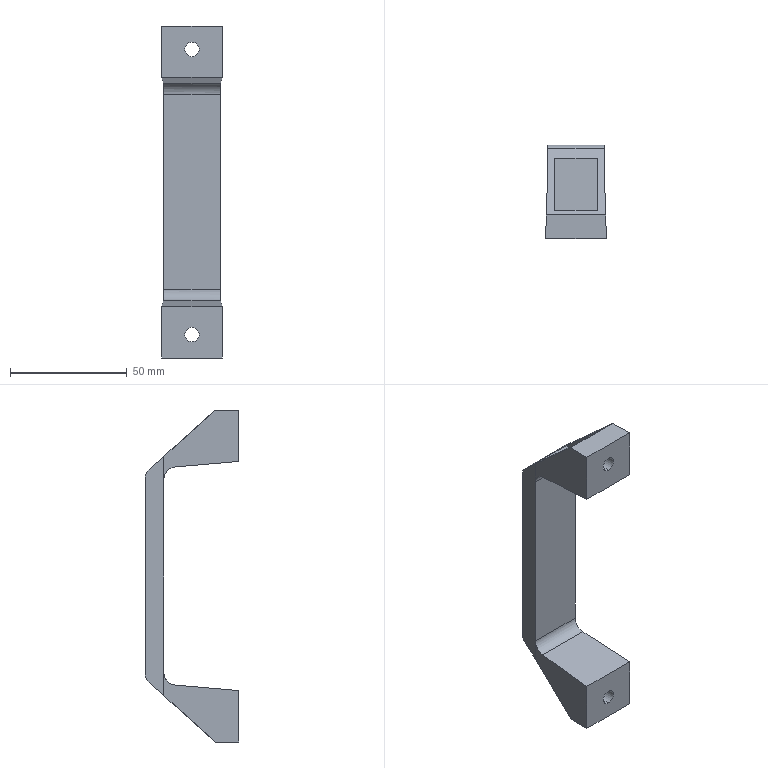Part | STEP file | 001-002-XAB31-L122 | 1 solid | 52 faces | box 26 x 40 x 142 mm | volume 36384 mm3 | plane 40 | cylinder 12 | commonest cylinder face diameters 6.2 x4 10 x4 13 x4